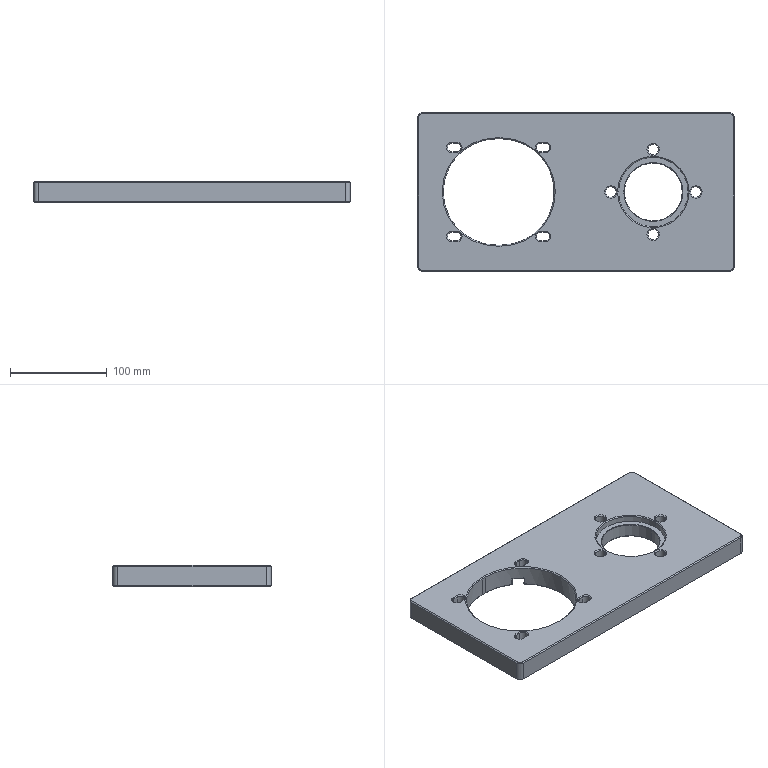Part | 1 solid | 244 faces | box 328 x 164 x 22 mm | volume 857509 mm3 | cone 108 | plane 69 | cylinder 67 | commonest cylinder face diameters 9 x12 2 x10 13.2 x10 3.3 x8 11 x8 18 x8